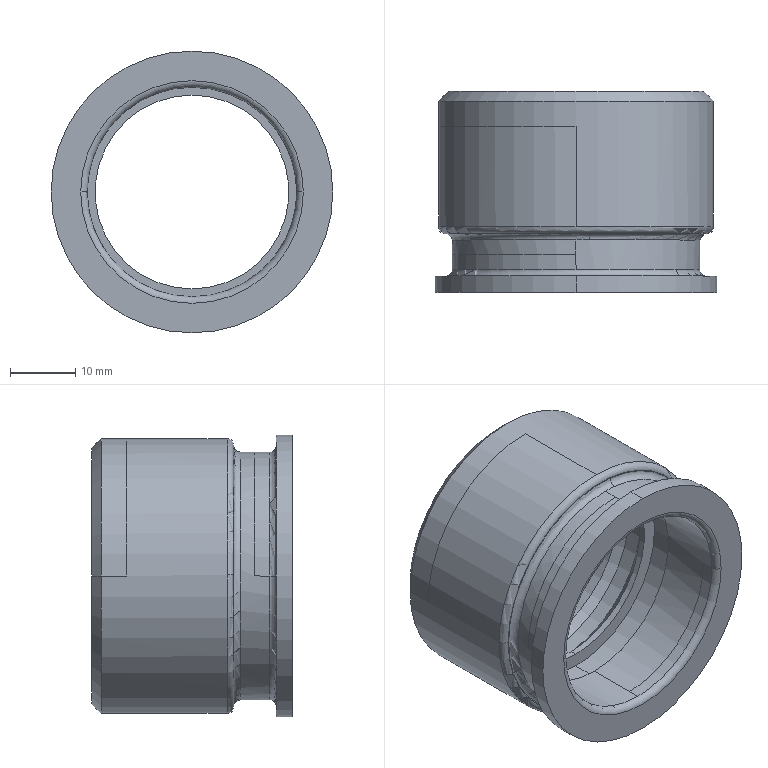Part | STEP file | 1 solid | 40 faces | box 43 x 30.7 x 43 mm | volume 14945 mm3 | cylinder 20 | torus 8 | plane 6 | cone 6 | commonest cylinder face diameters 32 x4 37.8 x4 29.614 x2 32.9 x2 34.014 x2 34.614 x2
STEP:
#1=CARTESIAN_POINT('',(0.,0.,0.));
#2=DIRECTION('',(0.,0.,1.));
#3=DIRECTION('',(1.,0.,0.));
#4=AXIS2_PLACEMENT_3D('',#1,#2,#3);
#5=CARTESIAN_POINT('',(-16.45,24.,-14.365));
#6=VERTEX_POINT('',#5);
#7=CARTESIAN_POINT('',(0.000000196,24.,2.085));
#8=VERTEX_POINT('',#7);
#9=CARTESIAN_POINT('',(0.000000196,24.,-14.365));
#10=DIRECTION('',(0.,1.,0.));
#11=DIRECTION('',(-1.,0.,0.));
#12=AXIS2_PLACEMENT_3D('',#9,#10,#11);
#13=CIRCLE('',#12,16.45);
#14=EDGE_CURVE('',#6,#8,#13,.T.);
#15=ORIENTED_EDGE('',*,*,#14,.F.);
#16=CARTESIAN_POINT('',(-16.45,27.9,-14.365));
#17=VERTEX_POINT('',#16);
#18=CARTESIAN_POINT('',(-16.45,24.,-14.365));
#19=DIRECTION('',(0.,1.,0.));
#20=VECTOR('',#19,3.9);
#21=LINE('',#18,#20);
#22=EDGE_CURVE('',#6,#17,#21,.T.);
#23=ORIENTED_EDGE('',*,*,#22,.T.);
#24=CARTESIAN_POINT('',(0.000000196,27.9,-30.815));
#25=VERTEX_POINT('',#24);
#26=CARTESIAN_POINT('',(0.000000196,27.9,-14.365));
#27=DIRECTION('',(0.,1.,0.));
#28=DIRECTION('',(0.,0.,-1.));
#29=AXIS2_PLACEMENT_3D('',#26,#27,#28);
#30=CIRCLE('',#29,16.45);
#31=EDGE_CURVE('',#25,#17,#30,.T.);
#32=ORIENTED_EDGE('',*,*,#31,.F.);
#33=CARTESIAN_POINT('',(16.45,27.9,-14.365));
#34=VERTEX_POINT('',#33);
#35=CARTESIAN_POINT('',(0.000000196,27.9,-14.365));
#36=DIRECTION('',(0.,1.,0.));
#37=DIRECTION('',(1.,0.,0.));
#38=AXIS2_PLACEMENT_3D('',#35,#36,#37);
#39=CIRCLE('',#38,16.45);
#40=EDGE_CURVE('',#34,#25,#39,.T.);
#41=ORIENTED_EDGE('',*,*,#40,.F.);
#42=CARTESIAN_POINT('',(16.45,24.,-14.365));
#43=VERTEX_POINT('',#42);
#44=CARTESIAN_POINT('',(16.45,24.,-14.365));
#45=DIRECTION('',(0.,1.,0.));
#46=VECTOR('',#45,3.9);
#47=LINE('',#44,#46);
#48=EDGE_CURVE('',#43,#34,#47,.T.);
#49=ORIENTED_EDGE('',*,*,#48,.F.);
#50=CARTESIAN_POINT('',(0.000000196,24.,-30.815));
#51=VERTEX_POINT('',#50);
#52=CARTESIAN_POINT('',(0.000000196,24.,-14.365));
#53=DIRECTION('',(0.,1.,0.));
#54=DIRECTION('',(1.,0.,0.));
#55=AXIS2_PLACEMENT_3D('',#52,#53,#54);
#56=CIRCLE('',#55,16.45);
#57=EDGE_CURVE('',#43,#51,#56,.T.);
#58=ORIENTED_EDGE('',*,*,#57,.T.);
#59=CARTESIAN_POINT('',(0.000000196,18.833,-30.815));
#60=VERTEX_POINT('',#59);
#61=CARTESIAN_POINT('',(0.000000196,24.,-30.815));
#62=DIRECTION('',(0.,-1.,0.000000118));
#63=VECTOR('',#62,5.167);
#64=LINE('',#61,#63);
#65=EDGE_CURVE('',#51,#60,#64,.T.);
#66=ORIENTED_EDGE('',*,*,#65,.T.);
#67=CARTESIAN_POINT('',(-16.45,18.833,-14.365));
#68=VERTEX_POINT('',#67);
#69=CARTESIAN_POINT('',(0.,18.833,-14.365));
#70=DIRECTION('',(0.,-1.,0.));
#71=DIRECTION('',(-1.,0.,0.));
#72=AXIS2_PLACEMENT_3D('',#69,#70,#71);
#73=CIRCLE('',#72,16.45);
#74=EDGE_CURVE('',#68,#60,#73,.T.);
#75=ORIENTED_EDGE('',*,*,#74,.F.);
#76=CARTESIAN_POINT('',(0.000000196,18.833,2.085));
#77=VERTEX_POINT('',#76);
#78=CARTESIAN_POINT('',(0.,18.833,-14.365));
#79=DIRECTION('',(0.,-1.,0.));
#80=DIRECTION('',(0.000000012,0.,1.));
#81=AXIS2_PLACEMENT_3D('',#78,#79,#80);
#82=CIRCLE('',#81,16.45);
#83=EDGE_CURVE('',#77,#68,#82,.T.);
#84=ORIENTED_EDGE('',*,*,#83,.F.);
#85=CARTESIAN_POINT('',(0.000000196,24.,2.085));
#86=DIRECTION('',(0.,-1.,0.000000024));
#87=VECTOR('',#86,5.167);
#88=LINE('',#85,#87);
#89=EDGE_CURVE('',#8,#77,#88,.T.);
#90=ORIENTED_EDGE('',*,*,#89,.F.);
#91=EDGE_LOOP('',(#15,#23,#32,#41,#49,#58,#66,#75,#84,#90));
#92=FACE_OUTER_BOUND('',#91,.F.);
#93=CARTESIAN_POINT('',(0.000000196,24.,-14.365));
#94=DIRECTION('',(0.,1.,0.));
#95=DIRECTION('',(0.,0.,1.));
#96=AXIS2_PLACEMENT_3D('',#93,#94,#95);
#97=CYLINDRICAL_SURFACE('',#96,16.45);
#98=ADVANCED_FACE('',(#92),#97,.F.);
#99=ORIENTED_EDGE('',*,*,#57,.F.);
#100=ORIENTED_EDGE('',*,*,#48,.T.);
#101=CARTESIAN_POINT('',(0.000000196,27.9,2.085));
#102=VERTEX_POINT('',#101);
#103=CARTESIAN_POINT('',(0.000000196,27.9,-14.365));
#104=DIRECTION('',(0.,1.,0.));
#105=DIRECTION('',(0.,0.,1.));
#106=AXIS2_PLACEMENT_3D('',#103,#104,#105);
#107=CIRCLE('',#106,16.45);
#108=EDGE_CURVE('',#102,#34,#107,.T.);
#109=ORIENTED_EDGE('',*,*,#108,.F.);
#110=CARTESIAN_POINT('',(0.000000196,27.9,-14.365));
#111=DIRECTION('',(0.,1.,0.));
#112=DIRECTION('',(-1.,0.,0.));
#113=AXIS2_PLACEMENT_3D('',#110,#111,#112);
#114=CIRCLE('',#113,16.45);
#115=EDGE_CURVE('',#17,#102,#114,.T.);
#116=ORIENTED_EDGE('',*,*,#115,.F.);
#117=ORIENTED_EDGE('',*,*,#22,.F.);
#118=ORIENTED_EDGE('',*,*,#14,.T.);
#119=ORIENTED_EDGE('',*,*,#89,.T.);
#120=CARTESIAN_POINT('',(16.45,18.833,-14.365));
#121=VERTEX_POINT('',#120);
#122=CARTESIAN_POINT('',(0.,18.833,-14.365));
#123=DIRECTION('',(0.,-1.,0.));
#124=DIRECTION('',(1.,0.,0.));
#125=AXIS2_PLACEMENT_3D('',#122,#123,#124);
#126=CIRCLE('',#125,16.45);
#127=EDGE_CURVE('',#121,#77,#126,.T.);
#128=ORIENTED_EDGE('',*,*,#127,.F.);
#129=CARTESIAN_POINT('',(0.,18.833,-14.365));
#130=DIRECTION('',(0.,-1.,0.));
#131=DIRECTION('',(0.000000012,0.,-1.));
#132=AXIS2_PLACEMENT_3D('',#129,#130,#131);
#133=CIRCLE('',#132,16.45);
#134=EDGE_CURVE('',#60,#121,#133,.T.);
#135=ORIENTED_EDGE('',*,*,#134,.F.);
#136=ORIENTED_EDGE('',*,*,#65,.F.);
#137=EDGE_LOOP('',(#99,#100,#109,#116,#117,#118,#119,#128,#135,#136));
#138=FACE_OUTER_BOUND('',#137,.F.);
#139=CARTESIAN_POINT('',(0.000000196,24.,-14.365));
#140=DIRECTION('',(0.,1.,0.));
#141=DIRECTION('',(0.,0.,1.));
#142=AXIS2_PLACEMENT_3D('',#139,#140,#141);
#143=CYLINDRICAL_SURFACE('',#142,16.45);
#144=ADVANCED_FACE('',(#138),#143,.F.);
#145=CARTESIAN_POINT('',(19.5,27.9,-14.365));
#146=VERTEX_POINT('',#145);
#147=CARTESIAN_POINT('',(0.,27.9,5.135));
#148=VERTEX_POINT('',#147);
#149=CARTESIAN_POINT('',(0.,27.9,-14.365));
#150=DIRECTION('',(0.,-1.,0.));
#151=DIRECTION('',(1.,0.,0.));
#152=AXIS2_PLACEMENT_3D('',#149,#150,#151);
#153=CIRCLE('',#152,19.5);
#154=EDGE_CURVE('',#146,#148,#153,.T.);
#155=ORIENTED_EDGE('',*,*,#154,.T.);
#156=CARTESIAN_POINT('',(-19.5,27.9,-14.365));
#157=VERTEX_POINT('',#156);
#158=CARTESIAN_POINT('',(0.,27.9,-14.365));
#159=DIRECTION('',(0.,-1.,0.));
#160=DIRECTION('',(0.,0.,1.));
#161=AXIS2_PLACEMENT_3D('',#158,#159,#160);
#162=CIRCLE('',#161,19.5);
#163=EDGE_CURVE('',#148,#157,#162,.T.);
#164=ORIENTED_EDGE('',*,*,#163,.T.);
#165=CARTESIAN_POINT('',(0.,27.9,-33.865));
#166=VERTEX_POINT('',#165);
#167=CARTESIAN_POINT('',(0.,27.9,-14.365));
#168=DIRECTION('',(0.,-1.,0.));
#169=DIRECTION('',(-1.,0.,0.));
#170=AXIS2_PLACEMENT_3D('',#167,#168,#169);
#171=CIRCLE('',#170,19.5);
#172=EDGE_CURVE('',#157,#166,#171,.T.);
#173=ORIENTED_EDGE('',*,*,#172,.T.);
#174=CARTESIAN_POINT('',(0.,27.9,-14.365));
#175=DIRECTION('',(0.,-1.,0.));
#176=DIRECTION('',(0.,0.,-1.));
#177=AXIS2_PLACEMENT_3D('',#174,#175,#176);
#178=CIRCLE('',#177,19.5);
#179=EDGE_CURVE('',#166,#146,#178,.T.);
#180=ORIENTED_EDGE('',*,*,#179,.T.);
#181=EDGE_LOOP('',(#155,#164,#173,#180));
#182=FACE_OUTER_BOUND('',#181,.F.);
#183=ORIENTED_EDGE('',*,*,#40,.T.);
#184=ORIENTED_EDGE('',*,*,#31,.T.);
#185=ORIENTED_EDGE('',*,*,#115,.T.);
#186=ORIENTED_EDGE('',*,*,#108,.T.);
#187=EDGE_LOOP('',(#183,#184,#185,#186));
#188=FACE_BOUND('',#187,.F.);
#189=CARTESIAN_POINT('',(0.,27.9,0.));
#190=DIRECTION('',(0.,1.,0.));
#191=DIRECTION('',(-1.,0.,0.));
#192=AXIS2_PLACEMENT_3D('',#189,#190,#191);
#193=PLANE('',#192);
#194=ADVANCED_FACE('',(#182,#188),#193,.T.);
#195=ORIENTED_EDGE('',*,*,#163,.F.);
#196=ORIENTED_EDGE('',*,*,#154,.F.);
#197=CARTESIAN_POINT('',(21.,26.4,-14.365));
#198=VERTEX_POINT('',#197);
#199=CARTESIAN_POINT('',(19.5,27.9,-14.365));
#200=DIRECTION('',(0.7071,-0.7071,0.000000001));
#201=VECTOR('',#200,2.121);
#202=LINE('',#199,#201);
#203=EDGE_CURVE('',#146,#198,#202,.T.);
#204=ORIENTED_EDGE('',*,*,#203,.T.);
#205=CARTESIAN_POINT('',(0.,26.4,6.635));
#206=VERTEX_POINT('',#205);
#207=CARTESIAN_POINT('',(0.,26.4,-14.365));
#208=DIRECTION('',(0.,-1.,0.));
#209=DIRECTION('',(1.,0.,0.));
#210=AXIS2_PLACEMENT_3D('',#207,#208,#209);
#211=CIRCLE('',#210,21.);
#212=EDGE_CURVE('',#198,#206,#211,.T.);
#213=ORIENTED_EDGE('',*,*,#212,.T.);
#214=CARTESIAN_POINT('',(-21.,26.4,-14.365));
#215=VERTEX_POINT('',#214);
#216=CARTESIAN_POINT('',(0.,26.4,-14.365));
#217=DIRECTION('',(0.,-1.,0.));
#218=DIRECTION('',(0.,0.,1.));
#219=AXIS2_PLACEMENT_3D('',#216,#217,#218);
#220=CIRCLE('',#219,21.);
#221=EDGE_CURVE('',#206,#215,#220,.T.);
#222=ORIENTED_EDGE('',*,*,#221,.T.);
#223=CARTESIAN_POINT('',(-19.5,27.9,-14.365));
#224=DIRECTION('',(-0.7071,-0.7071,-0.000000001));
#225=VECTOR('',#224,2.121);
#226=LINE('',#223,#225);
#227=EDGE_CURVE('',#157,#215,#226,.T.);
#228=ORIENTED_EDGE('',*,*,#227,.F.);
#229=EDGE_LOOP('',(#195,#196,#204,#213,#222,#228));
#230=FACE_OUTER_BOUND('',#229,.F.);
#231=CARTESIAN_POINT('',(0.,27.15,-14.365));
#232=DIRECTION('',(0.,-1.,0.));
#233=DIRECTION('',(0.,0.,-1.));
#234=AXIS2_PLACEMENT_3D('',#231,#232,#233);
#235=CONICAL_SURFACE('',#234,20.25,45.);
#236=ADVANCED_FACE('',(#230),#235,.T.);
#237=ORIENTED_EDGE('',*,*,#179,.F.);
#238=ORIENTED_EDGE('',*,*,#172,.F.);
#239=ORIENTED_EDGE('',*,*,#227,.T.);
#240=CARTESIAN_POINT('',(0.,26.4,-35.365));
#241=VERTEX_POINT('',#240);
#242=CARTESIAN_POINT('',(0.,26.4,-14.365));
#243=DIRECTION('',(0.,-1.,0.));
#244=DIRECTION('',(-1.,0.,0.));
#245=AXIS2_PLACEMENT_3D('',#242,#243,#244);
#246=CIRCLE('',#245,21.);
#247=EDGE_CURVE('',#215,#241,#246,.T.);
#248=ORIENTED_EDGE('',*,*,#247,.T.);
#249=CARTESIAN_POINT('',(0.,26.4,-14.365));
#250=DIRECTION('',(0.,-1.,0.));
#251=DIRECTION('',(0.,0.,-1.));
#252=AXIS2_PLACEMENT_3D('',#249,#250,#251);
#253=CIRCLE('',#252,21.);
#254=EDGE_CURVE('',#241,#198,#253,.T.);
#255=ORIENTED_EDGE('',*,*,#254,.T.);
#256=ORIENTED_EDGE('',*,*,#203,.F.);
#257=EDGE_LOOP('',(#237,#238,#239,#248,#255,#256));
#258=FACE_OUTER_BOUND('',#257,.F.);
#259=CARTESIAN_POINT('',(0.,27.15,-14.365));
#260=DIRECTION('',(0.,-1.,0.));
#261=DIRECTION('',(0.,0.,-1.));
#262=AXIS2_PLACEMENT_3D('',#259,#260,#261);
#263=CONICAL_SURFACE('',#262,20.25,45.);
#264=ADVANCED_FACE('',(#258),#263,.T.);
#265=ORIENTED_EDGE('',*,*,#254,.F.);
#266=ORIENTED_EDGE('',*,*,#247,.F.);
#267=CARTESIAN_POINT('',(-21.,22.5,-14.365));
#268=VERTEX_POINT('',#267);
#269=CARTESIAN_POINT('',(-21.,22.5,-14.365));
#270=DIRECTION('',(0.,1.,0.));
#271=VECTOR('',#270,3.9);
#272=LINE('',#269,#271);
#273=EDGE_CURVE('',#268,#215,#272,.T.);
#274=ORIENTED_EDGE('',*,*,#273,.F.);
#275=CARTESIAN_POINT('',(0.,22.5,6.635));
#276=VERTEX_POINT('',#275);
#277=CARTESIAN_POINT('',(0.,22.5,-14.365));
#278=DIRECTION('',(0.,-1.,0.));
#279=DIRECTION('',(0.,0.,1.));
#280=AXIS2_PLACEMENT_3D('',#277,#278,#279);
#281=CIRCLE('',#280,21.);
#282=EDGE_CURVE('',#276,#268,#281,.T.);
#283=ORIENTED_EDGE('',*,*,#282,.F.);
#284=CARTESIAN_POINT('',(0.,7.198,6.635));
#285=VERTEX_POINT('',#284);
#286=CARTESIAN_POINT('',(0.,22.5,6.635));
#287=DIRECTION('',(0.,-1.,0.));
#288=VECTOR('',#287,15.302);
#289=LINE('',#286,#288);
#290=EDGE_CURVE('',#276,#285,#289,.T.);
#291=ORIENTED_EDGE('',*,*,#290,.T.);
#292=CARTESIAN_POINT('',(-20.999,7.198,-14.197));
#293=VERTEX_POINT('',#292);
#294=CARTESIAN_POINT('',(0.,7.198,-14.365));
#295=DIRECTION('',(0.,1.,0.));
#296=DIRECTION('',(-1.,0.,0.008018));
#297=AXIS2_PLACEMENT_3D('',#294,#295,#296);
#298=CIRCLE('',#297,21.);
#299=EDGE_CURVE('',#293,#285,#298,.T.);
#300=ORIENTED_EDGE('',*,*,#299,.F.);
#301=CARTESIAN_POINT('',(0.,7.198,-35.365));
#302=VERTEX_POINT('',#301);
#303=CARTESIAN_POINT('',(0.,7.198,-14.365));
#304=DIRECTION('',(0.,1.,0.));
#305=DIRECTION('',(0.,0.,-1.));
#306=AXIS2_PLACEMENT_3D('',#303,#304,#305);
#307=CIRCLE('',#306,21.);
#308=EDGE_CURVE('',#302,#293,#307,.T.);
#309=ORIENTED_EDGE('',*,*,#308,.F.);
#310=CARTESIAN_POINT('',(0.,22.5,-35.365));
#311=VERTEX_POINT('',#310);
#312=CARTESIAN_POINT('',(0.,22.5,-35.365));
#313=DIRECTION('',(0.,-1.,0.));
#314=VECTOR('',#313,15.302);
#315=LINE('',#312,#314);
#316=EDGE_CURVE('',#311,#302,#315,.T.);
#317=ORIENTED_EDGE('',*,*,#316,.F.);
#318=CARTESIAN_POINT('',(21.,22.5,-14.365));
#319=VERTEX_POINT('',#318);
#320=CARTESIAN_POINT('',(0.,22.5,-14.365));
#321=DIRECTION('',(0.,1.,0.));
#322=DIRECTION('',(1.,0.,0.));
#323=AXIS2_PLACEMENT_3D('',#320,#321,#322);
#324=CIRCLE('',#323,21.);
#325=EDGE_CURVE('',#319,#311,#324,.T.);
#326=ORIENTED_EDGE('',*,*,#325,.F.);
#327=CARTESIAN_POINT('',(21.,22.5,-14.365));
#328=DIRECTION('',(0.,1.,0.));
#329=VECTOR('',#328,3.9);
#330=LINE('',#327,#329);
#331=EDGE_CURVE('',#319,#198,#330,.T.);
#332=ORIENTED_EDGE('',*,*,#331,.T.);
#333=EDGE_LOOP('',(#265,#266,#274,#283,#291,#300,#309,#317,#326,#332));
#334=FACE_OUTER_BOUND('',#333,.F.);
#335=CARTESIAN_POINT('',(0.,27.,-14.365));
#336=DIRECTION('',(0.,1.,0.));
#337=DIRECTION('',(0.,0.,1.));
#338=AXIS2_PLACEMENT_3D('',#335,#336,#337);
#339=CYLINDRICAL_SURFACE('',#338,21.);
#340=ADVANCED_FACE('',(#334),#339,.T.);
#341=ORIENTED_EDGE('',*,*,#221,.F.);
#342=ORIENTED_EDGE('',*,*,#212,.F.);
#343=ORIENTED_EDGE('',*,*,#331,.F.);
#344=ORIENTED_EDGE('',*,*,#325,.T.);
#345=ORIENTED_EDGE('',*,*,#316,.T.);
#346=CARTESIAN_POINT('',(20.999,7.198,-14.534));
#347=VERTEX_POINT('',#346);
#348=CARTESIAN_POINT('',(0.,7.198,-14.365));
#349=DIRECTION('',(0.,1.,0.));
#350=DIRECTION('',(1.,0.,-0.008018));
#351=AXIS2_PLACEMENT_3D('',#348,#349,#350);
#352=CIRCLE('',#351,21.);
#353=EDGE_CURVE('',#347,#302,#352,.T.);
#354=ORIENTED_EDGE('',*,*,#353,.F.);
#355=CARTESIAN_POINT('',(0.,7.198,-14.365));
#356=DIRECTION('',(0.,1.,0.));
#357=DIRECTION('',(0.,0.,1.));
#358=AXIS2_PLACEMENT_3D('',#355,#356,#357);
#359=CIRCLE('',#358,21.);
#360=EDGE_CURVE('',#285,#347,#359,.T.);
#361=ORIENTED_EDGE('',*,*,#360,.F.);
#362=ORIENTED_EDGE('',*,*,#290,.F.);
#363=ORIENTED_EDGE('',*,*,#282,.T.);
#364=ORIENTED_EDGE('',*,*,#273,.T.);
#365=EDGE_LOOP('',(#341,#342,#343,#344,#345,#354,#361,#362,#363,#364));
#366=FACE_OUTER_BOUND('',#365,.F.);
#367=CARTESIAN_POINT('',(0.,27.,-14.365));
#368=DIRECTION('',(0.,1.,0.));
#369=DIRECTION('',(0.,0.,1.));
#370=AXIS2_PLACEMENT_3D('',#367,#368,#369);
#371=CYLINDRICAL_SURFACE('',#370,21.);
#372=ADVANCED_FACE('',(#366),#371,.T.);
#373=ORIENTED_EDGE('',*,*,#353,.T.);
#374=ORIENTED_EDGE('',*,*,#308,.T.);
#375=CARTESIAN_POINT('',(-19.999,6.198,-14.205));
#376=VERTEX_POINT('',#375);
#377=CARTESIAN_POINT('',(-19.999,7.198,-14.205));
#378=DIRECTION('',(-0.008018,0.,-1.));
#379=DIRECTION('',(-0.000000415,-1.,0.000000003));
#380=AXIS2_PLACEMENT_3D('',#377,#378,#379);
#381=CIRCLE('',#380,1.);
#382=EDGE_CURVE('',#376,#293,#381,.T.);
#383=ORIENTED_EDGE('',*,*,#382,.F.);
#384=CARTESIAN_POINT('',(-20.,6.198,-14.365));
#385=VERTEX_POINT('',#384);
#386=CARTESIAN_POINT('',(0.,6.198,-14.365));
#387=DIRECTION('',(0.,-1.,0.));
#388=DIRECTION('',(-1.,0.,0.008018));
#389=AXIS2_PLACEMENT_3D('',#386,#387,#388);
#390=CIRCLE('',#389,20.);
#391=EDGE_CURVE('',#376,#385,#390,.T.);
#392=ORIENTED_EDGE('',*,*,#391,.T.);
#393=CARTESIAN_POINT('',(19.999,6.198,-14.526));
#394=VERTEX_POINT('',#393);
#395=CARTESIAN_POINT('',(0.,6.198,-14.365));
#396=DIRECTION('',(0.,1.,0.));
#397=DIRECTION('',(1.,0.,-0.008018));
#398=AXIS2_PLACEMENT_3D('',#395,#396,#397);
#399=CIRCLE('',#398,20.);
#400=EDGE_CURVE('',#394,#385,#399,.T.);
#401=ORIENTED_EDGE('',*,*,#400,.F.);
#402=CARTESIAN_POINT('',(19.999,7.198,-14.526));
#403=DIRECTION('',(0.008018,0.,1.));
#404=DIRECTION('',(0.000000415,-1.,-0.000000003));
#405=AXIS2_PLACEMENT_3D('',#402,#403,#404);
#406=CIRCLE('',#405,1.);
#407=EDGE_CURVE('',#394,#347,#406,.T.);
#408=ORIENTED_EDGE('',*,*,#407,.T.);
#409=EDGE_LOOP('',(#373,#374,#383,#392,#401,#408));
#410=FACE_OUTER_BOUND('',#409,.F.);
#411=CARTESIAN_POINT('',(0.,7.198,-14.365));
#412=DIRECTION('',(0.,-1.,0.));
#413=DIRECTION('',(1.,0.,-0.008018));
#414=AXIS2_PLACEMENT_3D('',#411,#412,#413);
#415=TOROIDAL_SURFACE('',#414,20.,1.);
#416=ADVANCED_FACE('',(#410),#415,.T.);
#417=ORIENTED_EDGE('',*,*,#407,.F.);
#418=CARTESIAN_POINT('',(20.,6.198,-14.365));
#419=VERTEX_POINT('',#418);
#420=CARTESIAN_POINT('',(0.,6.198,-14.365));
#421=DIRECTION('',(0.,-1.,0.));
#422=DIRECTION('',(1.,0.,-0.008018));
#423=AXIS2_PLACEMENT_3D('',#420,#421,#422);
#424=CIRCLE('',#423,20.);
#425=EDGE_CURVE('',#394,#419,#424,.T.);
#426=ORIENTED_EDGE('',*,*,#425,.T.);
#427=CARTESIAN_POINT('',(0.,6.198,-14.365));
#428=DIRECTION('',(0.,1.,0.));
#429=DIRECTION('',(-1.,0.,0.008018));
#430=AXIS2_PLACEMENT_3D('',#427,#428,#429);
#431=CIRCLE('',#430,20.);
#432=EDGE_CURVE('',#376,#419,#431,.T.);
#433=ORIENTED_EDGE('',*,*,#432,.F.);
#434=ORIENTED_EDGE('',*,*,#382,.T.);
#435=ORIENTED_EDGE('',*,*,#299,.T.);
#436=ORIENTED_EDGE('',*,*,#360,.T.);
#437=EDGE_LOOP('',(#417,#426,#433,#434,#435,#436));
#438=FACE_OUTER_BOUND('',#437,.F.);
#439=CARTESIAN_POINT('',(0.,7.198,-14.365));
#440=DIRECTION('',(0.,-1.,0.));
#441=DIRECTION('',(-1.,0.,0.008018));
#442=AXIS2_PLACEMENT_3D('',#439,#440,#441);
#443=TOROIDAL_SURFACE('',#442,20.,1.);
#444=ADVANCED_FACE('',(#438),#443,.T.);
#445=ORIENTED_EDGE('',*,*,#391,.F.);
#446=ORIENTED_EDGE('',*,*,#432,.T.);
#447=ORIENTED_EDGE('',*,*,#425,.F.);
#448=ORIENTED_EDGE('',*,*,#400,.T.);
#449=EDGE_LOOP('',(#445,#446,#447,#448));
#450=FACE_OUTER_BOUND('',#449,.F.);
#451=CARTESIAN_POINT('',(-2.091,6.198,-34.155));
#452=VERTEX_POINT('',#451);
#453=CARTESIAN_POINT('',(2.091,6.198,5.425));
#454=VERTEX_POINT('',#453);
#455=CARTESIAN_POINT('',(0.,6.198,-14.365));
#456=DIRECTION('',(0.,-1.,0.));
#457=DIRECTION('',(-0.1051,0.,-0.9945));
#458=AXIS2_PLACEMENT_3D('',#455,#456,#457);
#459=CIRCLE('',#458,19.9);
#460=EDGE_CURVE('',#452,#454,#459,.T.);
#461=ORIENTED_EDGE('',*,*,#460,.T.);
#462=CARTESIAN_POINT('',(1.718,6.198,5.46));
#463=VERTEX_POINT('',#462);
#464=CARTESIAN_POINT('',(0.,6.198,-14.365));
#465=DIRECTION('',(0.,-1.,0.));
#466=DIRECTION('',(0.1051,0.,0.9945));
#467=AXIS2_PLACEMENT_3D('',#464,#465,#466);
#468=CIRCLE('',#467,19.9);
#469=EDGE_CURVE('',#454,#463,#468,.T.);
#470=ORIENTED_EDGE('',*,*,#469,.T.);
#471=CARTESIAN_POINT('',(0.,6.198,-14.365));
#472=DIRECTION('',(0.,-1.,0.));
#473=DIRECTION('',(0.08631,0.,0.9963));
#474=AXIS2_PLACEMENT_3D('',#471,#472,#473);
#475=CIRCLE('',#474,19.9);
#476=EDGE_CURVE('',#463,#452,#475,.T.);
#477=ORIENTED_EDGE('',*,*,#476,.T.);
#478=EDGE_LOOP('',(#461,#470,#477));
#479=FACE_BOUND('',#478,.F.);
#480=CARTESIAN_POINT('',(0.,6.198,-14.365));
#481=DIRECTION('',(0.,1.,0.));
#482=DIRECTION('',(0.,0.,1.));
#483=AXIS2_PLACEMENT_3D('',#480,#481,#482);
#484=PLANE('',#483);
#485=ADVANCED_FACE('',(#450,#479),#484,.F.);
#486=CARTESIAN_POINT('',(-1.986,5.198,-33.161));
#487=VERTEX_POINT('',#486);
#488=CARTESIAN_POINT('',(0.000000011,5.198,-33.265));
#489=VERTEX_POINT('',#488);
#490=CARTESIAN_POINT('',(0.,5.198,-14.365));
#491=DIRECTION('',(0.,-1.,0.));
#492=DIRECTION('',(-0.1051,0.,-0.9945));
#493=AXIS2_PLACEMENT_3D('',#490,#491,#492);
#494=CIRCLE('',#493,18.9);
#495=EDGE_CURVE('',#487,#489,#494,.T.);
#496=ORIENTED_EDGE('',*,*,#495,.T.);
#497=CARTESIAN_POINT('',(1.986,5.198,4.43));
#498=VERTEX_POINT('',#497);
#499=CARTESIAN_POINT('',(0.,5.198,-14.365));
#500=DIRECTION('',(0.,-1.,0.));
#501=DIRECTION('',(-0.000000001,0.,-1.));
#502=AXIS2_PLACEMENT_3D('',#499,#500,#501);
#503=CIRCLE('',#502,18.9);
#504=EDGE_CURVE('',#489,#498,#503,.T.);
#505=ORIENTED_EDGE('',*,*,#504,.T.);
#506=CARTESIAN_POINT('',(2.091,5.198,5.425));
#507=DIRECTION('',(-0.9945,0.,0.1051));
#508=DIRECTION('',(-0.00001001,1.,-0.00009471));
#509=AXIS2_PLACEMENT_3D('',#506,#507,#508);
#510=CIRCLE('',#509,1.);
#511=EDGE_CURVE('',#454,#498,#510,.T.);
#512=ORIENTED_EDGE('',*,*,#511,.F.);
#513=ORIENTED_EDGE('',*,*,#460,.F.);
#514=CARTESIAN_POINT('',(-2.091,5.198,-34.155));
#515=DIRECTION('',(0.9945,0.,-0.1051));
#516=DIRECTION('',(0.000009728,1.,0.00009207));
#517=AXIS2_PLACEMENT_3D('',#514,#515,#516);
#518=CIRCLE('',#517,1.);
#519=EDGE_CURVE('',#452,#487,#518,.T.);
#520=ORIENTED_EDGE('',*,*,#519,.T.);
#521=EDGE_LOOP('',(#496,#505,#512,#513,#520));
#522=FACE_OUTER_BOUND('',#521,.F.);
#523=CARTESIAN_POINT('',(0.,5.198,-14.365));
#524=DIRECTION('',(0.,1.,0.));
#525=DIRECTION('',(0.1051,0.,0.9945));
#526=AXIS2_PLACEMENT_3D('',#523,#524,#525);
#527=TOROIDAL_SURFACE('',#526,19.9,1.);
#528=ADVANCED_FACE('',(#522),#527,.F.);
#529=CARTESIAN_POINT('',(-0.000004326,3.,4.535));
#530=VERTEX_POINT('',#529);
#531=CARTESIAN_POINT('',(-0.00001838,3.998,4.535));
#532=VERTEX_POINT('',#531);
#533=CARTESIAN_POINT('',(-0.000004326,3.,4.535));
#534=DIRECTION('',(-0.00001408,1.,0.000000017));
#535=VECTOR('',#534,0.9979);
#536=LINE('',#533,#535);
#537=EDGE_CURVE('',#530,#532,#536,.T.);
#538=ORIENTED_EDGE('',*,*,#537,.F.);
#539=CARTESIAN_POINT('',(-18.9,3.,-14.365));
#540=VERTEX_POINT('',#539);
#541=CARTESIAN_POINT('',(0.000000004,3.,-14.365));
#542=DIRECTION('',(-0.000000003,-1.,-0.000000016));
#543=DIRECTION('',(-0.000000543,-0.000000016,1.));
#544=AXIS2_PLACEMENT_3D('',#541,#542,#543);
#545=CIRCLE('',#544,18.9);
#546=EDGE_CURVE('',#530,#540,#545,.T.);
#547=ORIENTED_EDGE('',*,*,#546,.T.);
#548=CARTESIAN_POINT('',(-18.9,0.7,-14.365));
#549=VERTEX_POINT('',#548);
#550=CARTESIAN_POINT('',(-18.9,3.,-14.365));
#551=DIRECTION('',(0.,-1.,-0.000000017));
#552=VECTOR('',#551,2.3);
#553=LINE('',#550,#552);
#554=EDGE_CURVE('',#540,#549,#553,.T.);
#555=ORIENTED_EDGE('',*,*,#554,.T.);
#556=CARTESIAN_POINT('',(-0.000000002,0.7,-33.265));
#557=VERTEX_POINT('',#556);
#558=CARTESIAN_POINT('',(-0.000000002,0.7,-14.365));
#559=DIRECTION('',(0.000000003,1.,0.000000016));
#560=DIRECTION('',(0.,0.000000016,-1.));
#561=AXIS2_PLACEMENT_3D('',#558,#559,#560);
#562=CIRCLE('',#561,18.9);
#563=EDGE_CURVE('',#557,#549,#562,.T.);
#564=ORIENTED_EDGE('',*,*,#563,.F.);
#565=CARTESIAN_POINT('',(0.000000001,3.,-33.265));
#566=VERTEX_POINT('',#565);
#567=CARTESIAN_POINT('',(-0.000000002,0.7,-33.265));
#568=DIRECTION('',(0.000000002,1.,0.000000017));
#569=VECTOR('',#568,2.3);
#570=LINE('',#567,#569);
#571=EDGE_CURVE('',#557,#566,#570,.T.);
#572=ORIENTED_EDGE('',*,*,#571,.T.);
#573=CARTESIAN_POINT('',(0.000000001,3.,-33.265));
#574=DIRECTION('',(-0.000000001,1.,-0.00002785));
#575=VECTOR('',#574,2.198);
#576=LINE('',#573,#575);
#577=EDGE_CURVE('',#566,#489,#576,.T.);
#578=ORIENTED_EDGE('',*,*,#577,.T.);
#579=ORIENTED_EDGE('',*,*,#495,.F.);
#580=CARTESIAN_POINT('',(-0.0000265,5.198,4.535));
#581=VERTEX_POINT('',#580);
#582=CARTESIAN_POINT('',(0.,5.198,-14.365));
#583=DIRECTION('',(0.,-1.,0.));
#584=DIRECTION('',(-0.000001402,0.,1.));
#585=AXIS2_PLACEMENT_3D('',#582,#583,#584);
#586=CIRCLE('',#585,18.9);
#587=EDGE_CURVE('',#581,#487,#586,.T.);
#588=ORIENTED_EDGE('',*,*,#587,.F.);
#589=CARTESIAN_POINT('',(-0.00003302,5.198,4.535));
#590=DIRECTION('',(0.0000122,-1.,-0.00005101));
#591=VECTOR('',#590,1.2);
#592=LINE('',#589,#591);
#593=EDGE_CURVE('',#581,#532,#592,.T.);
#594=ORIENTED_EDGE('',*,*,#593,.T.);
#595=EDGE_LOOP('',(#538,#547,#555,#564,#572,#578,#579,#588,#594));
#596=FACE_OUTER_BOUND('',#595,.F.);
#597=CARTESIAN_POINT('',(0.000000008,4.096,-14.365));
#598=DIRECTION('',(-0.000000003,-1.,-0.000000016));
#599=DIRECTION('',(0.,0.000000016,-1.));
#600=AXIS2_PLACEMENT_3D('',#597,#598,#599);
#601=CYLINDRICAL_SURFACE('',#600,18.9);
#602=ADVANCED_FACE('',(#596),#601,.T.);
#603=CARTESIAN_POINT('',(1.631,5.198,4.464));
#604=VERTEX_POINT('',#603);
#605=CARTESIAN_POINT('',(0.,5.198,-14.365));
#606=DIRECTION('',(0.,-1.,0.));
#607=DIRECTION('',(0.08631,0.,0.9963));
#608=AXIS2_PLACEMENT_3D('',#605,#606,#607);
#609=CIRCLE('',#608,18.9);
#610=EDGE_CURVE('',#604,#581,#609,.T.);
#611=ORIENTED_EDGE('',*,*,#610,.F.);
#612=CARTESIAN_POINT('',(0.,5.198,-14.365));
#613=DIRECTION('',(0.,-1.,0.));
#614=DIRECTION('',(0.1051,0.,0.9945));
#615=AXIS2_PLACEMENT_3D('',#612,#613,#614);
#616=CIRCLE('',#615,18.9);
#617=EDGE_CURVE('',#498,#604,#616,.T.);
#618=ORIENTED_EDGE('',*,*,#617,.F.);
#619=ORIENTED_EDGE('',*,*,#504,.F.);
#620=ORIENTED_EDGE('',*,*,#577,.F.);
#621=CARTESIAN_POINT('',(18.9,3.,-14.365));
#622=VERTEX_POINT('',#621);
#623=CARTESIAN_POINT('',(0.000000004,3.,-14.365));
#624=DIRECTION('',(0.000000003,1.,0.000000016));
#625=DIRECTION('',(1.,-0.000000003,0.));
#626=AXIS2_PLACEMENT_3D('',#623,#624,#625);
#627=CIRCLE('',#626,18.9);
#628=EDGE_CURVE('',#622,#566,#627,.T.);
#629=ORIENTED_EDGE('',*,*,#628,.F.);
#630=CARTESIAN_POINT('',(18.9,0.7,-14.365));
#631=VERTEX_POINT('',#630);
#632=CARTESIAN_POINT('',(18.9,0.7,-14.365));
#633=DIRECTION('',(0.,1.,0.000000015));
#634=VECTOR('',#633,2.3);
#635=LINE('',#632,#634);
#636=EDGE_CURVE('',#631,#622,#635,.T.);
#637=ORIENTED_EDGE('',*,*,#636,.F.);
#638=CARTESIAN_POINT('',(0.000001606,0.7,4.535));
#639=VERTEX_POINT('',#638);
#640=CARTESIAN_POINT('',(0.000000002,0.7,-14.365));
#641=DIRECTION('',(-0.000000003,1.,0.000000016));
#642=DIRECTION('',(0.000000085,-0.000000016,1.));
#643=AXIS2_PLACEMENT_3D('',#640,#641,#642);
#644=CIRCLE('',#643,18.9);
#645=EDGE_CURVE('',#639,#631,#644,.T.);
#646=ORIENTED_EDGE('',*,*,#645,.F.);
#647=CARTESIAN_POINT('',(0.000001425,0.7,4.535));
#648=DIRECTION('',(-0.0000025,1.,0.000000017));
#649=VECTOR('',#648,2.3);
#650=LINE('',#647,#649);
#651=EDGE_CURVE('',#639,#530,#650,.T.);
#652=ORIENTED_EDGE('',*,*,#651,.T.);
#653=ORIENTED_EDGE('',*,*,#537,.T.);
#654=ORIENTED_EDGE('',*,*,#593,.F.);
#655=EDGE_LOOP('',(#611,#618,#619,#620,#629,#637,#646,#652,#653,#654));
#656=FACE_OUTER_BOUND('',#655,.F.);
#657=CARTESIAN_POINT('',(-0.000000008,4.096,-14.365));
#658=DIRECTION('',(0.000000003,-1.,-0.000000016));
#659=DIRECTION('',(0.,0.000000016,-1.));
#660=AXIS2_PLACEMENT_3D('',#657,#658,#659);
#661=CYLINDRICAL_SURFACE('',#660,18.9);
#662=ADVANCED_FACE('',(#656),#661,.T.);
#663=ORIENTED_EDGE('',*,*,#519,.F.);
#664=ORIENTED_EDGE('',*,*,#476,.F.);
#665=ORIENTED_EDGE('',*,*,#469,.F.);
#666=ORIENTED_EDGE('',*,*,#511,.T.);
#667=ORIENTED_EDGE('',*,*,#617,.T.);
#668=ORIENTED_EDGE('',*,*,#610,.T.);
#669=ORIENTED_EDGE('',*,*,#587,.T.);
#670=EDGE_LOOP('',(#663,#664,#665,#666,#667,#668,#669));
#671=FACE_OUTER_BOUND('',#670,.F.);
#672=CARTESIAN_POINT('',(0.,5.198,-14.365));
#673=DIRECTION('',(0.,1.,0.));
#674=DIRECTION('',(-0.08631,0.,-0.9963));
#675=AXIS2_PLACEMENT_3D('',#672,#673,#674);
#676=TOROIDAL_SURFACE('',#675,19.9,1.);
#677=ADVANCED_FACE('',(#671),#676,.F.);
#678=ORIENTED_EDGE('',*,*,#571,.F.);
#679=CARTESIAN_POINT('',(-0.000000002,0.7,-14.365));
#680=DIRECTION('',(0.000000003,1.,0.000000016));
#681=DIRECTION('',(1.,-0.000000003,0.));
#682=AXIS2_PLACEMENT_3D('',#679,#680,#681);
#683=CIRCLE('',#682,18.9);
#684=EDGE_CURVE('',#631,#557,#683,.T.);
#685=ORIENTED_EDGE('',*,*,#684,.F.);
#686=ORIENTED_EDGE('',*,*,#636,.T.);
#687=ORIENTED_EDGE('',*,*,#628,.T.);
#688=EDGE_LOOP('',(#678,#685,#686,#687));
#689=FACE_OUTER_BOUND('',#688,.F.);
#690=CARTESIAN_POINT('',(0.000000008,4.096,-14.365));
#691=DIRECTION('',(-0.000000003,-1.,-0.000000016));
#692=DIRECTION('',(0.,0.000000016,-1.));
#693=AXIS2_PLACEMENT_3D('',#690,#691,#692);
#694=CYLINDRICAL_SURFACE('',#693,18.9);
#695=ADVANCED_FACE('',(#689),#694,.T.);
#696=CARTESIAN_POINT('',(19.9,-0.3,-14.364));
#697=VERTEX_POINT('',#696);
#698=CARTESIAN_POINT('',(-19.9,-0.3,-14.365));
#699=VERTEX_POINT('',#698);
#700=CARTESIAN_POINT('',(-0.000000005,-0.3,-14.365));
#701=DIRECTION('',(0.000000003,1.,0.000000016));
#702=DIRECTION('',(1.,-0.000000003,0.00004702));
#703=AXIS2_PLACEMENT_3D('',#700,#701,#702);
#704=CIRCLE('',#703,19.9);
#705=EDGE_CURVE('',#697,#699,#704,.T.);
#706=ORIENTED_EDGE('',*,*,#705,.F.);
#707=CARTESIAN_POINT('',(19.9,0.7,-14.365));
#708=DIRECTION('',(0.,-0.000000016,1.));
#709=DIRECTION('',(-1.,-0.000000003,0.));
#710=AXIS2_PLACEMENT_3D('',#707,#708,#709);
#711=CIRCLE('',#710,1.);
#712=EDGE_CURVE('',#631,#697,#711,.T.);
#713=ORIENTED_EDGE('',*,*,#712,.F.);
#714=ORIENTED_EDGE('',*,*,#684,.T.);
#715=ORIENTED_EDGE('',*,*,#563,.T.);
#716=CARTESIAN_POINT('',(-19.9,0.7,-14.365));
#717=DIRECTION('',(0.,-0.000000016,1.));
#718=DIRECTION('',(-0.00007145,-1.,-0.000000016));
#719=AXIS2_PLACEMENT_3D('',#716,#717,#718);
#720=CIRCLE('',#719,1.);
#721=EDGE_CURVE('',#699,#549,#720,.T.);
#722=ORIENTED_EDGE('',*,*,#721,.F.);
#723=EDGE_LOOP('',(#706,#713,#714,#715,#722));
#724=FACE_OUTER_BOUND('',#723,.F.);
#725=CARTESIAN_POINT('',(-0.000000002,0.7,-14.365));
#726=DIRECTION('',(-0.000000003,-1.,-0.000000016));
#727=DIRECTION('',(-1.,0.000000003,0.));
#728=AXIS2_PLACEMENT_3D('',#725,#726,#727);
#729=TOROIDAL_SURFACE('',#728,19.9,1.);
#730=ADVANCED_FACE('',(#724),#729,.F.);
#731=CARTESIAN_POINT('',(-0.000000002,-0.3,-35.865));
#732=VERTEX_POINT('',#731);
#733=CARTESIAN_POINT('',(-0.000000002,-0.3,7.135));
#734=VERTEX_POINT('',#733);
#735=CARTESIAN_POINT('',(-0.000000002,-0.3,-14.365));
#736=DIRECTION('',(0.,-1.,0.));
#737=DIRECTION('',(0.,0.,-1.));
#738=AXIS2_PLACEMENT_3D('',#735,#736,#737);
#739=CIRCLE('',#738,21.5);
#740=EDGE_CURVE('',#732,#734,#739,.T.);
#741=ORIENTED_EDGE('',*,*,#740,.T.);
#742=CARTESIAN_POINT('',(-0.000000002,-0.3,-14.365));
#743=DIRECTION('',(0.,-1.,0.));
#744=DIRECTION('',(0.,0.,1.));
#745=AXIS2_PLACEMENT_3D('',#742,#743,#744);
#746=CIRCLE('',#745,21.5);
#747=EDGE_CURVE('',#734,#732,#746,.T.);
#748=ORIENTED_EDGE('',*,*,#747,.T.);
#749=EDGE_LOOP('',(#741,#748));
#750=FACE_OUTER_BOUND('',#749,.F.);
#751=ORIENTED_EDGE('',*,*,#705,.T.);
#752=CARTESIAN_POINT('',(0.000000005,-0.3,-14.365));
#753=DIRECTION('',(-0.000000003,1.,0.000000016));
#754=DIRECTION('',(-1.,-0.000000003,0.0000313));
#755=AXIS2_PLACEMENT_3D('',#752,#753,#754);
#756=CIRCLE('',#755,19.9);
#757=EDGE_CURVE('',#699,#697,#756,.T.);
#758=ORIENTED_EDGE('',*,*,#757,.T.);
#759=EDGE_LOOP('',(#751,#758));
#760=FACE_BOUND('',#759,.F.);
#761=CARTESIAN_POINT('',(0.,-0.3,0.));
#762=DIRECTION('',(0.,-1.,0.));
#763=DIRECTION('',(0.,0.,-1.));
#764=AXIS2_PLACEMENT_3D('',#761,#762,#763);
#765=PLANE('',#764);
#766=ADVANCED_FACE('',(#750,#760),#765,.F.);
#767=ORIENTED_EDGE('',*,*,#740,.F.);
#768=CARTESIAN_POINT('',(-0.000000002,-2.8,-35.865));
#769=VERTEX_POINT('',#768);
#770=CARTESIAN_POINT('',(-0.000000002,-2.8,-35.865));
#771=DIRECTION('',(0.,1.,0.));
#772=VECTOR('',#771,2.5);
#773=LINE('',#770,#772);
#774=EDGE_CURVE('',#769,#732,#773,.T.);
#775=ORIENTED_EDGE('',*,*,#774,.F.);
#776=CARTESIAN_POINT('',(-0.000000002,-2.8,7.135));
#777=VERTEX_POINT('',#776);
#778=CARTESIAN_POINT('',(-0.000000002,-2.8,-14.365));
#779=DIRECTION('',(0.,1.,0.));
#780=DIRECTION('',(0.,0.,1.));
#781=AXIS2_PLACEMENT_3D('',#778,#779,#780);
#782=CIRCLE('',#781,21.5);
#783=EDGE_CURVE('',#777,#769,#782,.T.);
#784=ORIENTED_EDGE('',*,*,#783,.F.);
#785=CARTESIAN_POINT('',(-0.000000002,-2.8,7.135));
#786=DIRECTION('',(0.,1.,0.));
#787=VECTOR('',#786,2.5);
#788=LINE('',#785,#787);
#789=EDGE_CURVE('',#777,#734,#788,.T.);
#790=ORIENTED_EDGE('',*,*,#789,.T.);
#791=EDGE_LOOP('',(#767,#775,#784,#790));
#792=FACE_OUTER_BOUND('',#791,.F.);
#793=CARTESIAN_POINT('',(-0.000000002,-0.3,-14.365));
#794=DIRECTION('',(0.,-1.,0.));
#795=DIRECTION('',(0.,0.,-1.));
#796=AXIS2_PLACEMENT_3D('',#793,#794,#795);
#797=CYLINDRICAL_SURFACE('',#796,21.5);
#798=ADVANCED_FACE('',(#792),#797,.T.);
#799=ORIENTED_EDGE('',*,*,#789,.F.);
#800=CARTESIAN_POINT('',(-0.000000002,-2.8,-14.365));
#801=DIRECTION('',(0.,1.,0.));
#802=DIRECTION('',(0.,0.,-1.));
#803=AXIS2_PLACEMENT_3D('',#800,#801,#802);
#804=CIRCLE('',#803,21.5);
#805=EDGE_CURVE('',#769,#777,#804,.T.);
#806=ORIENTED_EDGE('',*,*,#805,.F.);
#807=ORIENTED_EDGE('',*,*,#774,.T.);
#808=ORIENTED_EDGE('',*,*,#747,.F.);
#809=EDGE_LOOP('',(#799,#806,#807,#808));
#810=FACE_OUTER_BOUND('',#809,.F.);
#811=CARTESIAN_POINT('',(-0.000000002,-0.3,-14.365));
#812=DIRECTION('',(0.,-1.,0.));
#813=DIRECTION('',(0.,0.,-1.));
#814=AXIS2_PLACEMENT_3D('',#811,#812,#813);
#815=CYLINDRICAL_SURFACE('',#814,21.5);
#816=ADVANCED_FACE('',(#810),#815,.T.);
#817=ORIENTED_EDGE('',*,*,#805,.T.);
#818=ORIENTED_EDGE('',*,*,#783,.T.);
#819=EDGE_LOOP('',(#817,#818));
#820=FACE_OUTER_BOUND('',#819,.F.);
#821=CARTESIAN_POINT('',(-17.,-2.8,-14.366));
#822=VERTEX_POINT('',#821);
#823=CARTESIAN_POINT('',(17.,-2.8,-14.366));
#824=VERTEX_POINT('',#823);
#825=CARTESIAN_POINT('',(0.000000022,-2.8,-14.365));
#826=DIRECTION('',(0.000000008,-1.,0.000000054));
#827=DIRECTION('',(-1.,-0.000000008,-0.00002787));
#828=AXIS2_PLACEMENT_3D('',#825,#826,#827);
#829=CIRCLE('',#828,17.);
#830=EDGE_CURVE('',#822,#824,#829,.T.);
#831=ORIENTED_EDGE('',*,*,#830,.T.);
#832=CARTESIAN_POINT('',(-0.000000022,-2.8,-14.365));
#833=DIRECTION('',(-0.000000008,-1.,0.000000054));
#834=DIRECTION('',(1.,-0.000000008,-0.00004002));
#835=AXIS2_PLACEMENT_3D('',#832,#833,#834);
#836=CIRCLE('',#835,17.);
#837=EDGE_CURVE('',#824,#822,#836,.T.);
#838=ORIENTED_EDGE('',*,*,#837,.T.);
#839=EDGE_LOOP('',(#831,#838));
#840=FACE_BOUND('',#839,.F.);
#841=CARTESIAN_POINT('',(0.,-2.8,0.));
#842=DIRECTION('',(0.,-1.,0.));
#843=DIRECTION('',(0.,0.,-1.));
#844=AXIS2_PLACEMENT_3D('',#841,#842,#843);
#845=PLANE('',#844);
#846=ADVANCED_FACE('',(#820,#840),#845,.T.);
#847=CARTESIAN_POINT('',(-16.,-1.8,-14.365));
#848=VERTEX_POINT('',#847);
#849=CARTESIAN_POINT('',(-17.,-1.8,-14.365));
#850=DIRECTION('',(0.,-0.000000054,-1.));
#851=DIRECTION('',(1.,-0.000000008,0.));
#852=AXIS2_PLACEMENT_3D('',#849,#850,#851);
#853=CIRCLE('',#852,1.);
#854=EDGE_CURVE('',#848,#822,#853,.T.);
#855=ORIENTED_EDGE('',*,*,#854,.F.);
#856=CARTESIAN_POINT('',(-15.999,-1.8,-14.534));
#857=VERTEX_POINT('',#856);
#858=CARTESIAN_POINT('',(0.000000014,-1.8,-14.365));
#859=DIRECTION('',(0.000000008,-1.,0.000000054));
#860=DIRECTION('',(-1.,-0.000000008,-0.000000001));
#861=AXIS2_PLACEMENT_3D('',#858,#859,#860);
#862=CIRCLE('',#861,16.);
#863=EDGE_CURVE('',#848,#857,#862,.T.);
#864=ORIENTED_EDGE('',*,*,#863,.T.);
#865=CARTESIAN_POINT('',(0.000000014,-1.8,-30.365));
#866=VERTEX_POINT('',#865);
#867=CARTESIAN_POINT('',(0.000000014,-1.8,-14.365));
#868=DIRECTION('',(0.000000008,-1.,0.000000054));
#869=DIRECTION('',(-0.9999,-0.000000009,-0.01052));
#870=AXIS2_PLACEMENT_3D('',#867,#868,#869);
#871=CIRCLE('',#870,16.);
#872=EDGE_CURVE('',#857,#866,#871,.T.);
#873=ORIENTED_EDGE('',*,*,#872,.T.);
#874=CARTESIAN_POINT('',(16.,-1.8,-14.365));
#875=VERTEX_POINT('',#874);
#876=CARTESIAN_POINT('',(0.000000014,-1.8,-14.365));
#877=DIRECTION('',(0.000000008,-1.,0.000000054));
#878=DIRECTION('',(0.,-0.000000054,-1.));
#879=AXIS2_PLACEMENT_3D('',#876,#877,#878);
#880=CIRCLE('',#879,16.);
#881=EDGE_CURVE('',#866,#875,#880,.T.);
#882=ORIENTED_EDGE('',*,*,#881,.T.);
#883=CARTESIAN_POINT('',(17.,-1.8,-14.365));
#884=DIRECTION('',(0.,-0.000000054,-1.));
#885=DIRECTION('',(-0.00001426,-1.,0.000000054));
#886=AXIS2_PLACEMENT_3D('',#883,#884,#885);
#887=CIRCLE('',#886,1.);
#888=EDGE_CURVE('',#824,#875,#887,.T.);
#889=ORIENTED_EDGE('',*,*,#888,.F.);
#890=ORIENTED_EDGE('',*,*,#830,.F.);
#891=EDGE_LOOP('',(#855,#864,#873,#882,#889,#890));
#892=FACE_OUTER_BOUND('',#891,.F.);
#893=CARTESIAN_POINT('',(0.000000014,-1.8,-14.365));
#894=DIRECTION('',(0.000000008,-1.,0.000000054));
#895=DIRECTION('',(-1.,-0.000000008,0.));
#896=AXIS2_PLACEMENT_3D('',#893,#894,#895);
#897=TOROIDAL_SURFACE('',#896,17.,1.);
#898=ADVANCED_FACE('',(#892),#897,.T.);
#899=ORIENTED_EDGE('',*,*,#888,.T.);
#900=CARTESIAN_POINT('',(15.999,-1.8,-14.197));
#901=VERTEX_POINT('',#900);
#902=CARTESIAN_POINT('',(-0.000000014,-1.8,-14.365));
#903=DIRECTION('',(-0.000000008,-1.,0.000000054));
#904=DIRECTION('',(1.,-0.000000008,0.));
#905=AXIS2_PLACEMENT_3D('',#902,#903,#904);
#906=CIRCLE('',#905,16.);
#907=EDGE_CURVE('',#875,#901,#906,.T.);
#908=ORIENTED_EDGE('',*,*,#907,.T.);
#909=CARTESIAN_POINT('',(-0.000000008,-1.8,1.635));
#910=VERTEX_POINT('',#909);
#911=CARTESIAN_POINT('',(-0.000000014,-1.8,-14.365));
#912=DIRECTION('',(-0.000000008,-1.,0.000000054));
#913=DIRECTION('',(0.9999,-0.000000008,0.01052));
#914=AXIS2_PLACEMENT_3D('',#911,#912,#913);
#915=CIRCLE('',#914,16.);
#916=EDGE_CURVE('',#901,#910,#915,.T.);
#917=ORIENTED_EDGE('',*,*,#916,.T.);
#918=CARTESIAN_POINT('',(-0.000000014,-1.8,-14.365));
#919=DIRECTION('',(-0.000000008,-1.,0.000000054));
#920=DIRECTION('',(0.,0.000000054,1.));
#921=AXIS2_PLACEMENT_3D('',#918,#919,#920);
#922=CIRCLE('',#921,16.);
#923=EDGE_CURVE('',#910,#848,#922,.T.);
#924=ORIENTED_EDGE('',*,*,#923,.T.);
#925=ORIENTED_EDGE('',*,*,#854,.T.);
#926=ORIENTED_EDGE('',*,*,#837,.F.);
#927=EDGE_LOOP('',(#899,#908,#917,#924,#925,#926));
#928=FACE_OUTER_BOUND('',#927,.F.);
#929=CARTESIAN_POINT('',(-0.000000014,-1.8,-14.365));
#930=DIRECTION('',(-0.000000008,-1.,0.000000054));
#931=DIRECTION('',(1.,-0.000000008,0.));
#932=AXIS2_PLACEMENT_3D('',#929,#930,#931);
#933=TOROIDAL_SURFACE('',#932,17.,1.);
#934=ADVANCED_FACE('',(#928),#933,.T.);
#935=CARTESIAN_POINT('',(0.000000012,0.00000047,1.635));
#936=VERTEX_POINT('',#935);
#937=CARTESIAN_POINT('',(-0.000000007,-1.8,1.635));
#938=DIRECTION('',(0.00000001,1.,-0.000000054));
#939=VECTOR('',#938,1.8);
#940=LINE('',#937,#939);
#941=EDGE_CURVE('',#910,#936,#940,.T.);
#942=ORIENTED_EDGE('',*,*,#941,.F.);
#943=ORIENTED_EDGE('',*,*,#916,.F.);
#944=ORIENTED_EDGE('',*,*,#907,.F.);
#945=CARTESIAN_POINT('',(16.,0.000000565,-14.365));
#946=VERTEX_POINT('',#945);
#947=CARTESIAN_POINT('',(16.,0.000000565,-14.365));
#948=DIRECTION('',(0.,-1.,0.000000054));
#949=VECTOR('',#948,1.8);
#950=LINE('',#947,#949);
#951=EDGE_CURVE('',#946,#875,#950,.T.);
#952=ORIENTED_EDGE('',*,*,#951,.F.);
#953=CARTESIAN_POINT('',(-0.000000001,-0.000000387,-30.365));
#954=VERTEX_POINT('',#953);
#955=CARTESIAN_POINT('',(-0.000000001,0.000000481,-14.365));
#956=DIRECTION('',(0.000000008,-1.,0.000000054));
#957=DIRECTION('',(0.,-0.000000054,-1.));
#958=AXIS2_PLACEMENT_3D('',#955,#956,#957);
#959=CIRCLE('',#958,16.);
#960=EDGE_CURVE('',#954,#946,#959,.T.);
#961=ORIENTED_EDGE('',*,*,#960,.F.);
#962=CARTESIAN_POINT('',(0.,7.6,-30.365));
#963=VERTEX_POINT('',#962);
#964=CARTESIAN_POINT('',(0.,7.6,-30.365));
#965=DIRECTION('',(0.,-1.,0.000000054));
#966=VECTOR('',#965,7.6);
#967=LINE('',#964,#966);
#968=EDGE_CURVE('',#963,#954,#967,.T.);
#969=ORIENTED_EDGE('',*,*,#968,.F.);
#970=CARTESIAN_POINT('',(0.,7.6,1.635));
#971=VERTEX_POINT('',#970);
#972=CARTESIAN_POINT('',(0.000000062,7.6,-14.365));
#973=DIRECTION('',(0.000000008,1.,-0.000000054));
#974=DIRECTION('',(-0.000000004,0.000000054,1.));
#975=AXIS2_PLACEMENT_3D('',#972,#973,#974);
#976=CIRCLE('',#975,16.);
#977=EDGE_CURVE('',#971,#963,#976,.T.);
#978=ORIENTED_EDGE('',*,*,#977,.F.);
#979=CARTESIAN_POINT('',(0.000000012,0.00000047,1.635));
#980=DIRECTION('',(-0.000000001,1.,-0.000000054));
#981=VECTOR('',#980,7.6);
#982=LINE('',#979,#981);
#983=EDGE_CURVE('',#936,#971,#982,.T.);
#984=ORIENTED_EDGE('',*,*,#983,.F.);
#985=EDGE_LOOP('',(#942,#943,#944,#952,#961,#969,#978,#984));
#986=FACE_OUTER_BOUND('',#985,.F.);
#987=CARTESIAN_POINT('',(0.000000031,3.795,-14.365));
#988=DIRECTION('',(-0.000000008,-1.,0.000000054));
#989=DIRECTION('',(0.,-0.000000054,-1.));
#990=AXIS2_PLACEMENT_3D('',#987,#988,#989);
#991=CYLINDRICAL_SURFACE('',#990,16.);
#992=ADVANCED_FACE('',(#986),#991,.F.);
#993=CARTESIAN_POINT('',(-16.,-0.000000442,-14.365));
#994=VERTEX_POINT('',#993);
#995=CARTESIAN_POINT('',(-0.000000001,-0.000000312,-14.365));
#996=DIRECTION('',(-0.000000008,1.,-0.000000054));
#997=DIRECTION('',(-1.,-0.000000008,-0.000000001));
#998=AXIS2_PLACEMENT_3D('',#995,#996,#997);
#999=CIRCLE('',#998,16.);
#1000=EDGE_CURVE('',#994,#936,#999,.T.);
#1001=ORIENTED_EDGE('',*,*,#1000,.F.);
#1002=CARTESIAN_POINT('',(-16.,-1.8,-14.365));
#1003=DIRECTION('',(0.,1.,-0.000000058));
#1004=VECTOR('',#1003,1.8);
#1005=LINE('',#1002,#1004);
#1006=EDGE_CURVE('',#848,#994,#1005,.T.);
#1007=ORIENTED_EDGE('',*,*,#1006,.F.);
#1008=ORIENTED_EDGE('',*,*,#923,.F.);
#1009=ORIENTED_EDGE('',*,*,#941,.T.);
#1010=EDGE_LOOP('',(#1001,#1007,#1008,#1009));
#1011=FACE_OUTER_BOUND('',#1010,.F.);
#1012=CARTESIAN_POINT('',(0.000000031,3.795,-14.365));
#1013=DIRECTION('',(-0.000000008,-1.,0.000000054));
#1014=DIRECTION('',(0.,-0.000000054,-1.));
#1015=AXIS2_PLACEMENT_3D('',#1012,#1013,#1014);
#1016=CYLINDRICAL_SURFACE('',#1015,16.);
#1017=ADVANCED_FACE('',(#1011),#1016,.F.);
#1018=CARTESIAN_POINT('',(0.000000014,-1.8,-30.365));
#1019=DIRECTION('',(-0.000000008,1.,-0.000000054));
#1020=VECTOR('',#1019,1.8);
#1021=LINE('',#1018,#1020);
#1022=EDGE_CURVE('',#866,#954,#1021,.T.);
#1023=ORIENTED_EDGE('',*,*,#1022,.F.);
#1024=ORIENTED_EDGE('',*,*,#872,.F.);
#1025=ORIENTED_EDGE('',*,*,#863,.F.);
#1026=ORIENTED_EDGE('',*,*,#1006,.T.);
#1027=ORIENTED_EDGE('',*,*,#1000,.T.);
#1028=ORIENTED_EDGE('',*,*,#983,.T.);
#1029=CARTESIAN_POINT('',(-0.000000062,7.6,-14.365));
#1030=DIRECTION('',(-0.000000008,1.,-0.000000054));
#1031=DIRECTION('',(0.000000004,-0.000000054,-1.));
#1032=AXIS2_PLACEMENT_3D('',#1029,#1030,#1031);
#1033=CIRCLE('',#1032,16.);
#1034=EDGE_CURVE('',#963,#971,#1033,.T.);
#1035=ORIENTED_EDGE('',*,*,#1034,.F.);
#1036=ORIENTED_EDGE('',*,*,#968,.T.);
#1037=EDGE_LOOP('',(#1023,#1024,#1025,#1026,#1027,#1028,#1035,#1036));
#1038=FACE_OUTER_BOUND('',#1037,.F.);
#1039=CARTESIAN_POINT('',(-0.000000031,3.795,-14.365));
#1040=DIRECTION('',(0.000000008,-1.,0.000000054));
#1041=DIRECTION('',(0.,-0.000000054,-1.));
#1042=AXIS2_PLACEMENT_3D('',#1039,#1040,#1041);
#1043=CYLINDRICAL_SURFACE('',#1042,16.);
#1044=ADVANCED_FACE('',(#1038),#1043,.F.);
#1045=ORIENTED_EDGE('',*,*,#960,.T.);
#1046=ORIENTED_EDGE('',*,*,#951,.T.);
#1047=ORIENTED_EDGE('',*,*,#881,.F.);
#1048=ORIENTED_EDGE('',*,*,#1022,.T.);
#1049=EDGE_LOOP('',(#1045,#1046,#1047,#1048));
#1050=FACE_OUTER_BOUND('',#1049,.F.);
#1051=CARTESIAN_POINT('',(-0.000000031,3.795,-14.365));
#1052=DIRECTION('',(0.000000008,-1.,0.000000054));
#1053=DIRECTION('',(0.,-0.000000054,-1.));
#1054=AXIS2_PLACEMENT_3D('',#1051,#1052,#1053);
#1055=CYLINDRICAL_SURFACE('',#1054,16.);
#1056=ADVANCED_FACE('',(#1050),#1055,.F.);
#1057=CARTESIAN_POINT('',(0.,7.6,-31.372));
#1058=VERTEX_POINT('',#1057);
#1059=CARTESIAN_POINT('',(0.,7.6,2.642));
#1060=VERTEX_POINT('',#1059);
#1061=CARTESIAN_POINT('',(0.,7.6,-14.365));
#1062=DIRECTION('',(0.,-1.,0.));
#1063=DIRECTION('',(0.,0.,-1.));
#1064=AXIS2_PLACEMENT_3D('',#1061,#1062,#1063);
#1065=CIRCLE('',#1064,17.007);
#1066=EDGE_CURVE('',#1058,#1060,#1065,.T.);
#1067=ORIENTED_EDGE('',*,*,#1066,.T.);
#1068=CARTESIAN_POINT('',(0.,7.6,-14.365));
#1069=DIRECTION('',(0.,-1.,0.));
#1070=DIRECTION('',(0.,0.,1.));
#1071=AXIS2_PLACEMENT_3D('',#1068,#1069,#1070);
#1072=CIRCLE('',#1071,17.007);
#1073=EDGE_CURVE('',#1060,#1058,#1072,.T.);
#1074=ORIENTED_EDGE('',*,*,#1073,.T.);
#1075=EDGE_LOOP('',(#1067,#1074));
#1076=FACE_OUTER_BOUND('',#1075,.F.);
#1077=ORIENTED_EDGE('',*,*,#977,.T.);
#1078=ORIENTED_EDGE('',*,*,#1034,.T.);
#1079=EDGE_LOOP('',(#1077,#1078));
#1080=FACE_BOUND('',#1079,.F.);
#1081=CARTESIAN_POINT('',(0.,7.6,-14.365));
#1082=DIRECTION('',(0.,-1.,0.));
#1083=DIRECTION('',(0.,0.,-1.));
#1084=AXIS2_PLACEMENT_3D('',#1081,#1082,#1083);
#1085=PLANE('',#1084);
#1086=ADVANCED_FACE('',(#1076,#1080),#1085,.F.);
#1087=CARTESIAN_POINT('',(0.,11.6,-31.372));
#1088=VERTEX_POINT('',#1087);
#1089=CARTESIAN_POINT('',(0.,11.6,-31.372));
#1090=DIRECTION('',(0.,-1.,0.));
#1091=VECTOR('',#1090,4.);
#1092=LINE('',#1089,#1091);
#1093=EDGE_CURVE('',#1088,#1058,#1092,.T.);
#1094=ORIENTED_EDGE('',*,*,#1093,.F.);
#1095=CARTESIAN_POINT('',(0.,11.6,2.642));
#1096=VERTEX_POINT('',#1095);
#1097=CARTESIAN_POINT('',(0.,11.6,-14.365));
#1098=DIRECTION('',(0.,1.,0.));
#1099=DIRECTION('',(0.,0.,1.));
#1100=AXIS2_PLACEMENT_3D('',#1097,#1098,#1099);
#1101=CIRCLE('',#1100,17.007);
#1102=EDGE_CURVE('',#1096,#1088,#1101,.T.);
#1103=ORIENTED_EDGE('',*,*,#1102,.F.);
#1104=CARTESIAN_POINT('',(0.,11.6,2.642));
#1105=DIRECTION('',(0.,-1.,0.));
#1106=VECTOR('',#1105,4.);
#1107=LINE('',#1104,#1106);
#1108=EDGE_CURVE('',#1096,#1060,#1107,.T.);
#1109=ORIENTED_EDGE('',*,*,#1108,.T.);
#1110=ORIENTED_EDGE('',*,*,#1066,.F.);
#1111=EDGE_LOOP('',(#1094,#1103,#1109,#1110));
#1112=FACE_OUTER_BOUND('',#1111,.F.);
#1113=CARTESIAN_POINT('',(0.,19.994,-14.365));
#1114=DIRECTION('',(0.,1.,0.));
#1115=DIRECTION('',(0.,0.,1.));
#1116=AXIS2_PLACEMENT_3D('',#1113,#1114,#1115);
#1117=CYLINDRICAL_SURFACE('',#1116,17.007);
#1118=ADVANCED_FACE('',(#1112),#1117,.F.);
#1119=ORIENTED_EDGE('',*,*,#1073,.F.);
#1120=ORIENTED_EDGE('',*,*,#1108,.F.);
#1121=CARTESIAN_POINT('',(0.,11.6,-14.365));
#1122=DIRECTION('',(0.,1.,0.));
#1123=DIRECTION('',(0.,0.,-1.));
#1124=AXIS2_PLACEMENT_3D('',#1121,#1122,#1123);
#1125=CIRCLE('',#1124,17.007);
#1126=EDGE_CURVE('',#1088,#1096,#1125,.T.);
#1127=ORIENTED_EDGE('',*,*,#1126,.F.);
#1128=ORIENTED_EDGE('',*,*,#1093,.T.);
#1129=EDGE_LOOP('',(#1119,#1120,#1127,#1128));
#1130=FACE_OUTER_BOUND('',#1129,.F.);
#1131=CARTESIAN_POINT('',(0.,19.994,-14.365));
#1132=DIRECTION('',(0.,1.,0.));
#1133=DIRECTION('',(0.,0.,1.));
#1134=AXIS2_PLACEMENT_3D('',#1131,#1132,#1133);
#1135=CYLINDRICAL_SURFACE('',#1134,17.007);
#1136=ADVANCED_FACE('',(#1130),#1135,.F.);
#1137=ORIENTED_EDGE('',*,*,#1126,.T.);
#1138=ORIENTED_EDGE('',*,*,#1102,.T.);
#1139=EDGE_LOOP('',(#1137,#1138));
#1140=FACE_OUTER_BOUND('',#1139,.F.);
#1141=CARTESIAN_POINT('',(0.,11.6,-29.172));
#1142=VERTEX_POINT('',#1141);
#1143=CARTESIAN_POINT('',(0.,11.6,0.4415));
#1144=VERTEX_POINT('',#1143);
#1145=CARTESIAN_POINT('',(0.,11.6,-14.365));
#1146=DIRECTION('',(0.,-1.,0.));
#1147=DIRECTION('',(0.,0.,-1.));
#1148=AXIS2_PLACEMENT_3D('',#1145,#1146,#1147);
#1149=CIRCLE('',#1148,14.807);
#1150=EDGE_CURVE('',#1142,#1144,#1149,.T.);
#1151=ORIENTED_EDGE('',*,*,#1150,.T.);
#1152=CARTESIAN_POINT('',(0.,11.6,-14.365));
#1153=DIRECTION('',(0.,-1.,0.));
#1154=DIRECTION('',(0.,0.,1.));
#1155=AXIS2_PLACEMENT_3D('',#1152,#1153,#1154);
#1156=CIRCLE('',#1155,14.807);
#1157=EDGE_CURVE('',#1144,#1142,#1156,.T.);
#1158=ORIENTED_EDGE('',*,*,#1157,.T.);
#1159=EDGE_LOOP('',(#1151,#1158));
#1160=FACE_BOUND('',#1159,.F.);
#1161=CARTESIAN_POINT('',(0.,11.6,-14.365));
#1162=DIRECTION('',(0.,-1.,0.));
#1163=DIRECTION('',(0.,0.,-1.));
#1164=AXIS2_PLACEMENT_3D('',#1161,#1162,#1163);
#1165=PLANE('',#1164);
#1166=ADVANCED_FACE('',(#1140,#1160),#1165,.T.);
#1167=CARTESIAN_POINT('',(0.,12.6,-29.172));
#1168=VERTEX_POINT('',#1167);
#1169=CARTESIAN_POINT('',(0.,12.6,-29.172));
#1170=DIRECTION('',(0.,-1.,0.));
#1171=VECTOR('',#1170,1.);
#1172=LINE('',#1169,#1171);
#1173=EDGE_CURVE('',#1168,#1142,#1172,.T.);
#1174=ORIENTED_EDGE('',*,*,#1173,.F.);
#1175=CARTESIAN_POINT('',(0.,12.6,0.4415));
#1176=VERTEX_POINT('',#1175);
#1177=CARTESIAN_POINT('',(0.,12.6,-14.365));
#1178=DIRECTION('',(0.,1.,0.));
#1179=DIRECTION('',(0.,0.,1.));
#1180=AXIS2_PLACEMENT_3D('',#1177,#1178,#1179);
#1181=CIRCLE('',#1180,14.807);
#1182=EDGE_CURVE('',#1176,#1168,#1181,.T.);
#1183=ORIENTED_EDGE('',*,*,#1182,.F.);
#1184=CARTESIAN_POINT('',(0.,12.6,0.4415));
#1185=DIRECTION('',(0.,-1.,0.));
#1186=VECTOR('',#1185,1.);
#1187=LINE('',#1184,#1186);
#1188=EDGE_CURVE('',#1176,#1144,#1187,.T.);
#1189=ORIENTED_EDGE('',*,*,#1188,.T.);
#1190=ORIENTED_EDGE('',*,*,#1150,.F.);
#1191=EDGE_LOOP('',(#1174,#1183,#1189,#1190));
#1192=FACE_OUTER_BOUND('',#1191,.F.);
#1193=CARTESIAN_POINT('',(0.,25.952,-14.365));
#1194=DIRECTION('',(0.,1.,0.));
#1195=DIRECTION('',(0.,0.,1.));
#1196=AXIS2_PLACEMENT_3D('',#1193,#1194,#1195);
#1197=CYLINDRICAL_SURFACE('',#1196,14.807);
#1198=ADVANCED_FACE('',(#1192),#1197,.F.);
#1199=ORIENTED_EDGE('',*,*,#1157,.F.);
#1200=ORIENTED_EDGE('',*,*,#1188,.F.);
#1201=CARTESIAN_POINT('',(0.,12.6,-14.365));
#1202=DIRECTION('',(0.,1.,0.));
#1203=DIRECTION('',(0.,0.,-1.));
#1204=AXIS2_PLACEMENT_3D('',#1201,#1202,#1203);
#1205=CIRCLE('',#1204,14.807);
#1206=EDGE_CURVE('',#1168,#1176,#1205,.T.);
#1207=ORIENTED_EDGE('',*,*,#1206,.F.);
#1208=ORIENTED_EDGE('',*,*,#1173,.T.);
#1209=EDGE_LOOP('',(#1199,#1200,#1207,#1208));
#1210=FACE_OUTER_BOUND('',#1209,.F.);
#1211=CARTESIAN_POINT('',(0.,25.952,-14.365));
#1212=DIRECTION('',(0.,1.,0.));
#1213=DIRECTION('',(0.,0.,1.));
#1214=AXIS2_PLACEMENT_3D('',#1211,#1212,#1213);
#1215=CYLINDRICAL_SURFACE('',#1214,14.807);
#1216=ADVANCED_FACE('',(#1210),#1215,.F.);
#1217=ORIENTED_EDGE('',*,*,#1206,.T.);
#1218=CARTESIAN_POINT('',(0.,14.85,2.942));
#1219=VERTEX_POINT('',#1218);
#1220=CARTESIAN_POINT('',(0.,14.85,2.942));
#1221=DIRECTION('',(0.,-0.669,-0.7433));
#1222=VECTOR('',#1221,3.363);
#1223=LINE('',#1220,#1222);
#1224=EDGE_CURVE('',#1219,#1176,#1223,.T.);
#1225=ORIENTED_EDGE('',*,*,#1224,.F.);
#1226=CARTESIAN_POINT('',(0.,14.85,-31.672));
#1227=VERTEX_POINT('',#1226);
#1228=CARTESIAN_POINT('',(0.,14.85,-14.365));
#1229=DIRECTION('',(0.,-1.,0.));
#1230=DIRECTION('',(0.,0.,1.));
#1231=AXIS2_PLACEMENT_3D('',#1228,#1229,#1230);
#1232=CIRCLE('',#1231,17.307);
#1233=EDGE_CURVE('',#1219,#1227,#1232,.T.);
#1234=ORIENTED_EDGE('',*,*,#1233,.T.);
#1235=CARTESIAN_POINT('',(0.,14.85,-31.672));
#1236=DIRECTION('',(0.,-0.669,0.7433));
#1237=VECTOR('',#1236,3.363);
#1238=LINE('',#1235,#1237);
#1239=EDGE_CURVE('',#1227,#1168,#1238,.T.);
#1240=ORIENTED_EDGE('',*,*,#1239,.T.);
#1241=EDGE_LOOP('',(#1217,#1225,#1234,#1240));
#1242=FACE_OUTER_BOUND('',#1241,.F.);
#1243=CARTESIAN_POINT('',(0.,13.725,-14.365));
#1244=DIRECTION('',(0.,1.,0.));
#1245=DIRECTION('',(0.,0.,1.));
#1246=AXIS2_PLACEMENT_3D('',#1243,#1244,#1245);
#1247=CONICAL_SURFACE('',#1246,16.057,48.013);
#1248=ADVANCED_FACE('',(#1242),#1247,.F.);
#1249=ORIENTED_EDGE('',*,*,#1239,.F.);
#1250=CARTESIAN_POINT('',(0.,14.85,-14.365));
#1251=DIRECTION('',(0.,-1.,0.));
#1252=DIRECTION('',(0.,0.,-1.));
#1253=AXIS2_PLACEMENT_3D('',#1250,#1251,#1252);
#1254=CIRCLE('',#1253,17.307);
#1255=EDGE_CURVE('',#1227,#1219,#1254,.T.);
#1256=ORIENTED_EDGE('',*,*,#1255,.T.);
#1257=ORIENTED_EDGE('',*,*,#1224,.T.);
#1258=ORIENTED_EDGE('',*,*,#1182,.T.);
#1259=EDGE_LOOP('',(#1249,#1256,#1257,#1258));
#1260=FACE_OUTER_BOUND('',#1259,.F.);
#1261=CARTESIAN_POINT('',(0.,13.725,-14.365));
#1262=DIRECTION('',(0.,1.,0.));
#1263=DIRECTION('',(0.,0.,1.));
#1264=AXIS2_PLACEMENT_3D('',#1261,#1262,#1263);
#1265=CONICAL_SURFACE('',#1264,16.057,48.013);
#1266=ADVANCED_FACE('',(#1260),#1265,.F.);
#1267=CARTESIAN_POINT('',(0.,17.35,-31.672));
#1268=VERTEX_POINT('',#1267);
#1269=CARTESIAN_POINT('',(0.,17.35,-31.672));
#1270=DIRECTION('',(0.,-1.,0.));
#1271=VECTOR('',#1270,2.5);
#1272=LINE('',#1269,#1271);
#1273=EDGE_CURVE('',#1268,#1227,#1272,.T.);
#1274=ORIENTED_EDGE('',*,*,#1273,.F.);
#1275=CARTESIAN_POINT('',(17.307,17.35,-14.365));
#1276=VERTEX_POINT('',#1275);
#1277=CARTESIAN_POINT('',(0.,17.35,-14.365));
#1278=DIRECTION('',(0.,1.,0.));
#1279=DIRECTION('',(1.,0.,0.));
#1280=AXIS2_PLACEMENT_3D('',#1277,#1278,#1279);
#1281=CIRCLE('',#1280,17.307);
#1282=EDGE_CURVE('',#1276,#1268,#1281,.T.);
#1283=ORIENTED_EDGE('',*,*,#1282,.F.);
#1284=CARTESIAN_POINT('',(0.,17.35,2.942));
#1285=VERTEX_POINT('',#1284);
#1286=CARTESIAN_POINT('',(0.,17.35,-14.365));
#1287=DIRECTION('',(0.,1.,0.));
#1288=DIRECTION('',(0.,0.,1.));
#1289=AXIS2_PLACEMENT_3D('',#1286,#1287,#1288);
#1290=CIRCLE('',#1289,17.307);
#1291=EDGE_CURVE('',#1285,#1276,#1290,.T.);
#1292=ORIENTED_EDGE('',*,*,#1291,.F.);
#1293=CARTESIAN_POINT('',(0.,17.35,2.942));
#1294=DIRECTION('',(0.,-1.,0.));
#1295=VECTOR('',#1294,2.5);
#1296=LINE('',#1293,#1295);
#1297=EDGE_CURVE('',#1285,#1219,#1296,.T.);
#1298=ORIENTED_EDGE('',*,*,#1297,.T.);
#1299=ORIENTED_EDGE('',*,*,#1255,.F.);
#1300=EDGE_LOOP('',(#1274,#1283,#1292,#1298,#1299));
#1301=FACE_OUTER_BOUND('',#1300,.F.);
#1302=CARTESIAN_POINT('',(0.,19.994,-14.365));
#1303=DIRECTION('',(0.,1.,0.));
#1304=DIRECTION('',(0.,0.,1.));
#1305=AXIS2_PLACEMENT_3D('',#1302,#1303,#1304);
#1306=CYLINDRICAL_SURFACE('',#1305,17.307);
#1307=ADVANCED_FACE('',(#1301),#1306,.F.);
#1308=ORIENTED_EDGE('',*,*,#1233,.F.);
#1309=ORIENTED_EDGE('',*,*,#1297,.F.);
#1310=CARTESIAN_POINT('',(-17.307,17.35,-14.365));
#1311=VERTEX_POINT('',#1310);
#1312=CARTESIAN_POINT('',(0.,17.35,-14.365));
#1313=DIRECTION('',(0.,1.,0.));
#1314=DIRECTION('',(-1.,0.,0.));
#1315=AXIS2_PLACEMENT_3D('',#1312,#1313,#1314);
#1316=CIRCLE('',#1315,17.307);
#1317=EDGE_CURVE('',#1311,#1285,#1316,.T.);
#1318=ORIENTED_EDGE('',*,*,#1317,.F.);
#1319=CARTESIAN_POINT('',(0.,17.35,-14.365));
#1320=DIRECTION('',(0.,1.,0.));
#1321=DIRECTION('',(0.,0.,-1.));
#1322=AXIS2_PLACEMENT_3D('',#1319,#1320,#1321);
#1323=CIRCLE('',#1322,17.307);
#1324=EDGE_CURVE('',#1268,#1311,#1323,.T.);
#1325=ORIENTED_EDGE('',*,*,#1324,.F.);
#1326=ORIENTED_EDGE('',*,*,#1273,.T.);
#1327=EDGE_LOOP('',(#1308,#1309,#1318,#1325,#1326));
#1328=FACE_OUTER_BOUND('',#1327,.F.);
#1329=CARTESIAN_POINT('',(0.,19.994,-14.365));
#1330=DIRECTION('',(0.,1.,0.));
#1331=DIRECTION('',(0.,0.,1.));
#1332=AXIS2_PLACEMENT_3D('',#1329,#1330,#1331);
#1333=CYLINDRICAL_SURFACE('',#1332,17.307);
#1334=ADVANCED_FACE('',(#1328),#1333,.F.);
#1335=CARTESIAN_POINT('',(-17.307,17.35,-14.365));
#1336=DIRECTION('',(0.5003,0.8659,0.));
#1337=VECTOR('',#1336,1.713);
#1338=LINE('',#1335,#1337);
#1339=EDGE_CURVE('',#1311,#68,#1338,.T.);
#1340=ORIENTED_EDGE('',*,*,#1339,.F.);
#1341=ORIENTED_EDGE('',*,*,#1317,.T.);
#1342=ORIENTED_EDGE('',*,*,#1291,.T.);
#1343=CARTESIAN_POINT('',(17.307,17.35,-14.365));
#1344=DIRECTION('',(-0.5003,0.8659,0.));
#1345=VECTOR('',#1344,1.713);
#1346=LINE('',#1343,#1345);
#1347=EDGE_CURVE('',#1276,#121,#1346,.T.);
#1348=ORIENTED_EDGE('',*,*,#1347,.T.);
#1349=ORIENTED_EDGE('',*,*,#127,.T.);
#1350=ORIENTED_EDGE('',*,*,#83,.T.);
#1351=EDGE_LOOP('',(#1340,#1341,#1342,#1348,#1349,#1350));
#1352=FACE_OUTER_BOUND('',#1351,.F.);
#1353=CARTESIAN_POINT('',(0.,18.091,-14.365));
#1354=DIRECTION('',(0.,-1.,0.));
#1355=DIRECTION('',(1.,0.,0.));
#1356=AXIS2_PLACEMENT_3D('',#1353,#1354,#1355);
#1357=CONICAL_SURFACE('',#1356,16.878,30.018);
#1358=ADVANCED_FACE('',(#1352),#1357,.F.);
#1359=ORIENTED_EDGE('',*,*,#134,.T.);
#1360=ORIENTED_EDGE('',*,*,#1347,.F.);
#1361=ORIENTED_EDGE('',*,*,#1282,.T.);
#1362=ORIENTED_EDGE('',*,*,#1324,.T.);
#1363=ORIENTED_EDGE('',*,*,#1339,.T.);
#1364=ORIENTED_EDGE('',*,*,#74,.T.);
#1365=EDGE_LOOP('',(#1359,#1360,#1361,#1362,#1363,#1364));
#1366=FACE_OUTER_BOUND('',#1365,.F.);
#1367=CARTESIAN_POINT('',(0.,18.091,-14.365));
#1368=DIRECTION('',(0.,-1.,0.));
#1369=DIRECTION('',(1.,0.,0.));
#1370=AXIS2_PLACEMENT_3D('',#1367,#1368,#1369);
#1371=CONICAL_SURFACE('',#1370,16.878,30.018);
#1372=ADVANCED_FACE('',(#1366),#1371,.F.);
#1373=ORIENTED_EDGE('',*,*,#757,.F.);
#1374=ORIENTED_EDGE('',*,*,#721,.T.);
#1375=CARTESIAN_POINT('',(0.000000002,0.7,-14.365));
#1376=DIRECTION('',(-0.000000003,1.,0.000000016));
#1377=DIRECTION('',(-1.,-0.000000003,0.));
#1378=AXIS2_PLACEMENT_3D('',#1375,#1376,#1377);
#1379=CIRCLE('',#1378,18.9);
#1380=EDGE_CURVE('',#549,#639,#1379,.T.);
#1381=ORIENTED_EDGE('',*,*,#1380,.T.);
#1382=ORIENTED_EDGE('',*,*,#645,.T.);
#1383=ORIENTED_EDGE('',*,*,#712,.T.);
#1384=EDGE_LOOP('',(#1373,#1374,#1381,#1382,#1383));
#1385=FACE_OUTER_BOUND('',#1384,.F.);
#1386=CARTESIAN_POINT('',(0.000000002,0.7,-14.365));
#1387=DIRECTION('',(0.000000003,-1.,-0.000000016));
#1388=DIRECTION('',(1.,0.000000003,0.));
#1389=AXIS2_PLACEMENT_3D('',#1386,#1387,#1388);
#1390=TOROIDAL_SURFACE('',#1389,19.9,1.);
#1391=ADVANCED_FACE('',(#1385),#1390,.F.);
#1392=ORIENTED_EDGE('',*,*,#651,.F.);
#1393=ORIENTED_EDGE('',*,*,#1380,.F.);
#1394=ORIENTED_EDGE('',*,*,#554,.F.);
#1395=ORIENTED_EDGE('',*,*,#546,.F.);
#1396=EDGE_LOOP('',(#1392,#1393,#1394,#1395));
#1397=FACE_OUTER_BOUND('',#1396,.F.);
#1398=CARTESIAN_POINT('',(-0.000000008,4.096,-14.365));
#1399=DIRECTION('',(0.000000003,-1.,-0.000000016));
#1400=DIRECTION('',(0.,0.000000016,-1.));
#1401=AXIS2_PLACEMENT_3D('',#1398,#1399,#1400);
#1402=CYLINDRICAL_SURFACE('',#1401,18.9);
#1403=ADVANCED_FACE('',(#1397),#1402,.T.);
#1404=CLOSED_SHELL('',(#98,#144,#194,#236,#264,#340,#372,#416,#444,#485,#528,#602,#662,#677,#695,#730,#766,#798,#816,#846,#898,#934,#992,#1017,#1044,#1056,#1086,#1118,#1136,#1166,#1198,#1216,#1248,#1266,#1307,#1334,#1358,#1372,#1391,#1403));
#1405=MANIFOLD_SOLID_BREP('',#1404);
#1406=(LENGTH_UNIT()NAMED_UNIT(*)SI_UNIT(.MILLI.,.METRE.));
#1407=UNCERTAINTY_MEASURE_WITH_UNIT(LENGTH_MEASURE(0.006814),#1406,'','');
#1408=(NAMED_UNIT(*)PLANE_ANGLE_UNIT()SI_UNIT($,.RADIAN.));
#1409=PLANE_ANGLE_MEASURE_WITH_UNIT(PLANE_ANGLE_MEASURE(0.01745),#1408);
#1410=(CONVERSION_BASED_UNIT('DEGREE',#1409)NAMED_UNIT(*)PLANE_ANGLE_UNIT());
#1411=(NAMED_UNIT(*)SI_UNIT($,.STERADIAN.)SOLID_ANGLE_UNIT());
#1412=(GEOMETRIC_REPRESENTATION_CONTEXT(3)GLOBAL_UNCERTAINTY_ASSIGNED_CONTEXT((#1407))GLOBAL_UNIT_ASSIGNED_CONTEXT((#1406,#1410,#1411))REPRESENTATION_CONTEXT('',''));
#1413=ADVANCED_BREP_SHAPE_REPRESENTATION('',(#4,#1405),#1412);